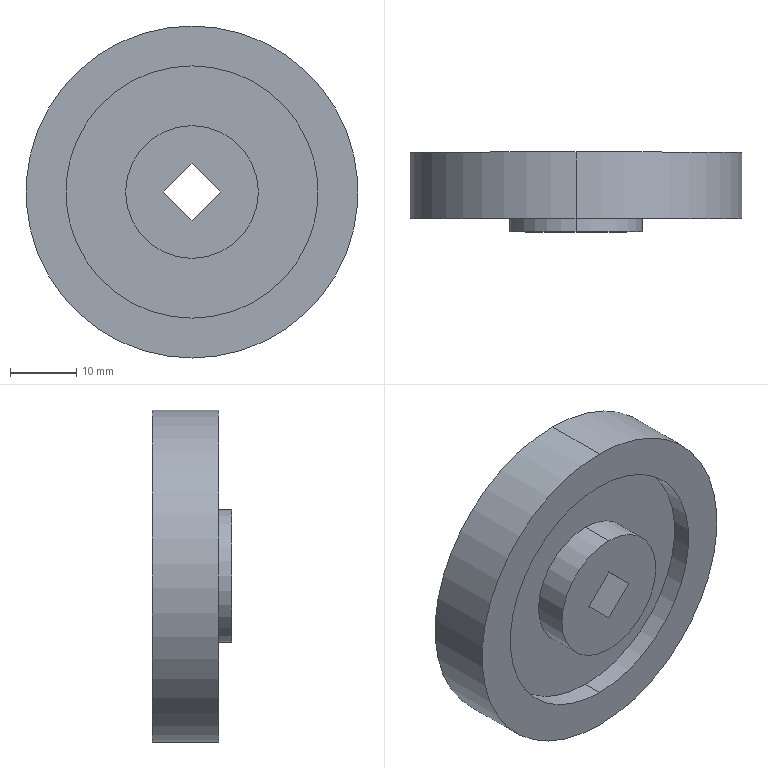Part | SolidWorks | features ICE 3, Extrusion 1 | 1 solid | 20 faces | box 50 x 12 x 50 mm | volume 14912 mm3 | cylinder 10 | plane 10 | commonest cylinder face diameters 20 x4 38 x4 50 x2
STEP:
#1=CARTESIAN_POINT('',(0.,2.,10.));
#2=VERTEX_POINT('',#1);
#3=CARTESIAN_POINT('',(0.,2.,-10.));
#4=VERTEX_POINT('',#3);
#5=CARTESIAN_POINT('',(0.,2.,0.));
#6=DIRECTION('',(0.,1.,0.));
#7=DIRECTION('',(0.,0.,1.));
#8=AXIS2_PLACEMENT_3D('',#5,#6,#7);
#9=CIRCLE('',#8,10.);
#10=EDGE_CURVE('',#2,#4,#9,.T.);
#11=ORIENTED_EDGE('',*,*,#10,.T.);
#12=CARTESIAN_POINT('',(0.,5.,-10.));
#13=VERTEX_POINT('',#12);
#14=CARTESIAN_POINT('',(0.,-7.,-10.));
#15=DIRECTION('',(0.,1.,0.));
#16=VECTOR('',#15,1000.);
#17=LINE('',#14,#16);
#18=EDGE_CURVE('',#4,#13,#17,.T.);
#19=ORIENTED_EDGE('',*,*,#18,.T.);
#20=CARTESIAN_POINT('',(0.,5.,10.));
#21=VERTEX_POINT('',#20);
#22=CARTESIAN_POINT('',(0.,5.,0.));
#23=DIRECTION('',(0.,1.,0.));
#24=DIRECTION('',(0.,0.,1.));
#25=AXIS2_PLACEMENT_3D('',#22,#23,#24);
#26=CIRCLE('',#25,10.);
#27=EDGE_CURVE('',#21,#13,#26,.T.);
#28=ORIENTED_EDGE('',*,*,#27,.F.);
#29=CARTESIAN_POINT('',(0.,-7.,10.));
#30=DIRECTION('',(0.,1.,0.));
#31=VECTOR('',#30,1000.);
#32=LINE('',#29,#31);
#33=EDGE_CURVE('',#2,#21,#32,.T.);
#34=ORIENTED_EDGE('',*,*,#33,.F.);
#35=EDGE_LOOP('',(#11,#19,#28,#34));
#36=FACE_OUTER_BOUND('',#35,.T.);
#37=CARTESIAN_POINT('',(0.,-7.,0.));
#38=DIRECTION('',(0.,1.,0.));
#39=DIRECTION('',(0.,0.,1.));
#40=AXIS2_PLACEMENT_3D('',#37,#38,#39);
#41=CYLINDRICAL_SURFACE('',#40,10.);
#42=ADVANCED_FACE('',(#36),#41,.T.);
#43=CARTESIAN_POINT('',(0.,-7.,10.));
#44=VERTEX_POINT('',#43);
#45=CARTESIAN_POINT('',(0.,-7.,-10.));
#46=VERTEX_POINT('',#45);
#47=CARTESIAN_POINT('',(0.,-7.,0.));
#48=DIRECTION('',(0.,1.,0.));
#49=DIRECTION('',(0.,0.,1.));
#50=AXIS2_PLACEMENT_3D('',#47,#48,#49);
#51=CIRCLE('',#50,10.);
#52=EDGE_CURVE('',#44,#46,#51,.T.);
#53=ORIENTED_EDGE('',*,*,#52,.T.);
#54=CARTESIAN_POINT('',(0.,-2.,-10.));
#55=VERTEX_POINT('',#54);
#56=CARTESIAN_POINT('',(0.,-7.,-10.));
#57=DIRECTION('',(0.,1.,0.));
#58=VECTOR('',#57,1000.);
#59=LINE('',#56,#58);
#60=EDGE_CURVE('',#46,#55,#59,.T.);
#61=ORIENTED_EDGE('',*,*,#60,.T.);
#62=CARTESIAN_POINT('',(0.,-2.,10.));
#63=VERTEX_POINT('',#62);
#64=CARTESIAN_POINT('',(0.,-2.,0.));
#65=DIRECTION('',(0.,1.,0.));
#66=DIRECTION('',(0.,0.,1.));
#67=AXIS2_PLACEMENT_3D('',#64,#65,#66);
#68=CIRCLE('',#67,10.);
#69=EDGE_CURVE('',#63,#55,#68,.T.);
#70=ORIENTED_EDGE('',*,*,#69,.F.);
#71=CARTESIAN_POINT('',(0.,-7.,10.));
#72=DIRECTION('',(0.,1.,0.));
#73=VECTOR('',#72,1000.);
#74=LINE('',#71,#73);
#75=EDGE_CURVE('',#44,#63,#74,.T.);
#76=ORIENTED_EDGE('',*,*,#75,.F.);
#77=EDGE_LOOP('',(#53,#61,#70,#76));
#78=FACE_OUTER_BOUND('',#77,.T.);
#79=CARTESIAN_POINT('',(0.,-7.,0.));
#80=DIRECTION('',(0.,1.,0.));
#81=DIRECTION('',(0.,0.,1.));
#82=AXIS2_PLACEMENT_3D('',#79,#80,#81);
#83=CYLINDRICAL_SURFACE('',#82,10.);
#84=ADVANCED_FACE('',(#78),#83,.T.);
#85=CARTESIAN_POINT('',(0.,5.,-19.));
#86=VERTEX_POINT('',#85);
#87=CARTESIAN_POINT('',(0.,5.,19.));
#88=VERTEX_POINT('',#87);
#89=CARTESIAN_POINT('',(0.,5.,0.));
#90=DIRECTION('',(0.,1.,0.));
#91=DIRECTION('',(0.,0.,1.));
#92=AXIS2_PLACEMENT_3D('',#89,#90,#91);
#93=CIRCLE('',#92,19.);
#94=EDGE_CURVE('',#86,#88,#93,.T.);
#95=ORIENTED_EDGE('',*,*,#94,.T.);
#96=CARTESIAN_POINT('',(0.,2.,19.));
#97=VERTEX_POINT('',#96);
#98=CARTESIAN_POINT('',(0.,5.,19.));
#99=DIRECTION('',(0.,-1.,0.));
#100=VECTOR('',#99,1000.);
#101=LINE('',#98,#100);
#102=EDGE_CURVE('',#88,#97,#101,.T.);
#103=ORIENTED_EDGE('',*,*,#102,.T.);
#104=CARTESIAN_POINT('',(0.,2.,-19.));
#105=VERTEX_POINT('',#104);
#106=CARTESIAN_POINT('',(0.,2.,0.));
#107=DIRECTION('',(0.,1.,0.));
#108=DIRECTION('',(0.,0.,1.));
#109=AXIS2_PLACEMENT_3D('',#106,#107,#108);
#110=CIRCLE('',#109,19.);
#111=EDGE_CURVE('',#105,#97,#110,.T.);
#112=ORIENTED_EDGE('',*,*,#111,.F.);
#113=CARTESIAN_POINT('',(0.,5.,-19.));
#114=DIRECTION('',(0.,-1.,0.));
#115=VECTOR('',#114,1000.);
#116=LINE('',#113,#115);
#117=EDGE_CURVE('',#86,#105,#116,.T.);
#118=ORIENTED_EDGE('',*,*,#117,.F.);
#119=EDGE_LOOP('',(#95,#103,#112,#118));
#120=FACE_OUTER_BOUND('',#119,.T.);
#121=CARTESIAN_POINT('',(0.,5.,0.));
#122=DIRECTION('',(0.,-1.,0.));
#123=DIRECTION('',(0.,0.,-1.));
#124=AXIS2_PLACEMENT_3D('',#121,#122,#123);
#125=CYLINDRICAL_SURFACE('',#124,19.);
#126=ADVANCED_FACE('',(#120),#125,.F.);
#127=CARTESIAN_POINT('',(0.,5.,25.));
#128=VERTEX_POINT('',#127);
#129=CARTESIAN_POINT('',(0.,5.,-25.));
#130=VERTEX_POINT('',#129);
#131=CARTESIAN_POINT('',(0.,5.,0.));
#132=DIRECTION('',(0.,1.,0.));
#133=DIRECTION('',(0.,0.,1.));
#134=AXIS2_PLACEMENT_3D('',#131,#132,#133);
#135=CIRCLE('',#134,25.);
#136=EDGE_CURVE('',#128,#130,#135,.T.);
#137=ORIENTED_EDGE('',*,*,#136,.F.);
#138=CARTESIAN_POINT('',(0.,-5.,25.));
#139=VERTEX_POINT('',#138);
#140=CARTESIAN_POINT('',(0.,5.,25.));
#141=DIRECTION('',(0.,-1.,0.));
#142=VECTOR('',#141,1000.);
#143=LINE('',#140,#142);
#144=EDGE_CURVE('',#128,#139,#143,.T.);
#145=ORIENTED_EDGE('',*,*,#144,.T.);
#146=CARTESIAN_POINT('',(0.,-5.,-25.));
#147=VERTEX_POINT('',#146);
#148=CARTESIAN_POINT('',(0.,-5.,0.));
#149=DIRECTION('',(0.,1.,0.));
#150=DIRECTION('',(0.,0.,1.));
#151=AXIS2_PLACEMENT_3D('',#148,#149,#150);
#152=CIRCLE('',#151,25.);
#153=EDGE_CURVE('',#139,#147,#152,.T.);
#154=ORIENTED_EDGE('',*,*,#153,.T.);
#155=CARTESIAN_POINT('',(0.,5.,-25.));
#156=DIRECTION('',(0.,-1.,0.));
#157=VECTOR('',#156,1000.);
#158=LINE('',#155,#157);
#159=EDGE_CURVE('',#130,#147,#158,.T.);
#160=ORIENTED_EDGE('',*,*,#159,.F.);
#161=EDGE_LOOP('',(#137,#145,#154,#160));
#162=FACE_OUTER_BOUND('',#161,.T.);
#163=CARTESIAN_POINT('',(0.,5.,0.));
#164=DIRECTION('',(0.,-1.,0.));
#165=DIRECTION('',(0.,0.,-1.));
#166=AXIS2_PLACEMENT_3D('',#163,#164,#165);
#167=CYLINDRICAL_SURFACE('',#166,25.);
#168=ADVANCED_FACE('',(#162),#167,.T.);
#169=CARTESIAN_POINT('',(0.,-2.,-19.));
#170=VERTEX_POINT('',#169);
#171=CARTESIAN_POINT('',(0.,-2.,19.));
#172=VERTEX_POINT('',#171);
#173=CARTESIAN_POINT('',(0.,-2.,0.));
#174=DIRECTION('',(0.,1.,0.));
#175=DIRECTION('',(0.,0.,1.));
#176=AXIS2_PLACEMENT_3D('',#173,#174,#175);
#177=CIRCLE('',#176,19.);
#178=EDGE_CURVE('',#170,#172,#177,.T.);
#179=ORIENTED_EDGE('',*,*,#178,.T.);
#180=CARTESIAN_POINT('',(0.,-5.,19.));
#181=VERTEX_POINT('',#180);
#182=CARTESIAN_POINT('',(0.,5.,19.));
#183=DIRECTION('',(0.,-1.,0.));
#184=VECTOR('',#183,1000.);
#185=LINE('',#182,#184);
#186=EDGE_CURVE('',#172,#181,#185,.T.);
#187=ORIENTED_EDGE('',*,*,#186,.T.);
#188=CARTESIAN_POINT('',(0.,-5.,-19.));
#189=VERTEX_POINT('',#188);
#190=CARTESIAN_POINT('',(0.,-5.,0.));
#191=DIRECTION('',(0.,1.,0.));
#192=DIRECTION('',(0.,0.,1.));
#193=AXIS2_PLACEMENT_3D('',#190,#191,#192);
#194=CIRCLE('',#193,19.);
#195=EDGE_CURVE('',#189,#181,#194,.T.);
#196=ORIENTED_EDGE('',*,*,#195,.F.);
#197=CARTESIAN_POINT('',(0.,5.,-19.));
#198=DIRECTION('',(0.,-1.,0.));
#199=VECTOR('',#198,1000.);
#200=LINE('',#197,#199);
#201=EDGE_CURVE('',#170,#189,#200,.T.);
#202=ORIENTED_EDGE('',*,*,#201,.F.);
#203=EDGE_LOOP('',(#179,#187,#196,#202));
#204=FACE_OUTER_BOUND('',#203,.T.);
#205=CARTESIAN_POINT('',(0.,5.,0.));
#206=DIRECTION('',(0.,-1.,0.));
#207=DIRECTION('',(0.,0.,-1.));
#208=AXIS2_PLACEMENT_3D('',#205,#206,#207);
#209=CYLINDRICAL_SURFACE('',#208,19.);
#210=ADVANCED_FACE('',(#204),#209,.F.);
#211=ORIENTED_EDGE('',*,*,#186,.F.);
#212=CARTESIAN_POINT('',(0.,-2.,0.));
#213=DIRECTION('',(0.,1.,0.));
#214=DIRECTION('',(0.,0.,1.));
#215=AXIS2_PLACEMENT_3D('',#212,#213,#214);
#216=CIRCLE('',#215,19.);
#217=EDGE_CURVE('',#172,#170,#216,.T.);
#218=ORIENTED_EDGE('',*,*,#217,.T.);
#219=ORIENTED_EDGE('',*,*,#201,.T.);
#220=CARTESIAN_POINT('',(0.,-5.,0.));
#221=DIRECTION('',(0.,1.,0.));
#222=DIRECTION('',(0.,0.,1.));
#223=AXIS2_PLACEMENT_3D('',#220,#221,#222);
#224=CIRCLE('',#223,19.);
#225=EDGE_CURVE('',#181,#189,#224,.T.);
#226=ORIENTED_EDGE('',*,*,#225,.F.);
#227=EDGE_LOOP('',(#211,#218,#219,#226));
#228=FACE_OUTER_BOUND('',#227,.T.);
#229=CARTESIAN_POINT('',(0.,5.,0.));
#230=DIRECTION('',(0.,-1.,0.));
#231=DIRECTION('',(0.,0.,-1.));
#232=AXIS2_PLACEMENT_3D('',#229,#230,#231);
#233=CYLINDRICAL_SURFACE('',#232,19.);
#234=ADVANCED_FACE('',(#228),#233,.F.);
#235=CARTESIAN_POINT('',(0.,5.,0.));
#236=DIRECTION('',(0.,1.,0.));
#237=DIRECTION('',(0.,0.,1.));
#238=AXIS2_PLACEMENT_3D('',#235,#236,#237);
#239=CIRCLE('',#238,25.);
#240=EDGE_CURVE('',#130,#128,#239,.T.);
#241=ORIENTED_EDGE('',*,*,#240,.T.);
#242=ORIENTED_EDGE('',*,*,#136,.T.);
#243=EDGE_LOOP('',(#241,#242));
#244=FACE_OUTER_BOUND('',#243,.T.);
#245=ORIENTED_EDGE('',*,*,#94,.F.);
#246=CARTESIAN_POINT('',(0.,5.,0.));
#247=DIRECTION('',(0.,1.,0.));
#248=DIRECTION('',(0.,0.,1.));
#249=AXIS2_PLACEMENT_3D('',#246,#247,#248);
#250=CIRCLE('',#249,19.);
#251=EDGE_CURVE('',#88,#86,#250,.T.);
#252=ORIENTED_EDGE('',*,*,#251,.F.);
#253=EDGE_LOOP('',(#245,#252));
#254=FACE_BOUND('',#253,.T.);
#255=CARTESIAN_POINT('',(0.,5.,0.));
#256=DIRECTION('',(0.,1.,0.));
#257=DIRECTION('',(0.,0.,1.));
#258=AXIS2_PLACEMENT_3D('',#255,#256,#257);
#259=PLANE('',#258);
#260=ADVANCED_FACE('',(#244,#254),#259,.T.);
#261=CARTESIAN_POINT('',(0.,-5.,0.));
#262=DIRECTION('',(0.,1.,0.));
#263=DIRECTION('',(0.,0.,1.));
#264=AXIS2_PLACEMENT_3D('',#261,#262,#263);
#265=CIRCLE('',#264,25.);
#266=EDGE_CURVE('',#147,#139,#265,.T.);
#267=ORIENTED_EDGE('',*,*,#266,.F.);
#268=ORIENTED_EDGE('',*,*,#153,.F.);
#269=EDGE_LOOP('',(#267,#268));
#270=FACE_OUTER_BOUND('',#269,.T.);
#271=ORIENTED_EDGE('',*,*,#195,.T.);
#272=ORIENTED_EDGE('',*,*,#225,.T.);
#273=EDGE_LOOP('',(#271,#272));
#274=FACE_BOUND('',#273,.T.);
#275=CARTESIAN_POINT('',(0.,-5.,0.));
#276=DIRECTION('',(0.,1.,0.));
#277=DIRECTION('',(0.,0.,1.));
#278=AXIS2_PLACEMENT_3D('',#275,#276,#277);
#279=PLANE('',#278);
#280=ADVANCED_FACE('',(#270,#274),#279,.F.);
#281=ORIENTED_EDGE('',*,*,#144,.F.);
#282=ORIENTED_EDGE('',*,*,#240,.F.);
#283=ORIENTED_EDGE('',*,*,#159,.T.);
#284=ORIENTED_EDGE('',*,*,#266,.T.);
#285=EDGE_LOOP('',(#281,#282,#283,#284));
#286=FACE_OUTER_BOUND('',#285,.T.);
#287=CARTESIAN_POINT('',(0.,5.,0.));
#288=DIRECTION('',(0.,-1.,0.));
#289=DIRECTION('',(0.,0.,-1.));
#290=AXIS2_PLACEMENT_3D('',#287,#288,#289);
#291=CYLINDRICAL_SURFACE('',#290,25.);
#292=ADVANCED_FACE('',(#286),#291,.T.);
#293=ORIENTED_EDGE('',*,*,#102,.F.);
#294=ORIENTED_EDGE('',*,*,#251,.T.);
#295=ORIENTED_EDGE('',*,*,#117,.T.);
#296=CARTESIAN_POINT('',(0.,2.,0.));
#297=DIRECTION('',(0.,1.,0.));
#298=DIRECTION('',(0.,0.,1.));
#299=AXIS2_PLACEMENT_3D('',#296,#297,#298);
#300=CIRCLE('',#299,19.);
#301=EDGE_CURVE('',#97,#105,#300,.T.);
#302=ORIENTED_EDGE('',*,*,#301,.F.);
#303=EDGE_LOOP('',(#293,#294,#295,#302));
#304=FACE_OUTER_BOUND('',#303,.T.);
#305=CARTESIAN_POINT('',(0.,5.,0.));
#306=DIRECTION('',(0.,-1.,0.));
#307=DIRECTION('',(0.,0.,-1.));
#308=AXIS2_PLACEMENT_3D('',#305,#306,#307);
#309=CYLINDRICAL_SURFACE('',#308,19.);
#310=ADVANCED_FACE('',(#304),#309,.F.);
#311=ORIENTED_EDGE('',*,*,#111,.T.);
#312=ORIENTED_EDGE('',*,*,#301,.T.);
#313=EDGE_LOOP('',(#311,#312));
#314=FACE_OUTER_BOUND('',#313,.T.);
#315=ORIENTED_EDGE('',*,*,#10,.F.);
#316=CARTESIAN_POINT('',(0.,2.,0.));
#317=DIRECTION('',(0.,1.,0.));
#318=DIRECTION('',(0.,0.,1.));
#319=AXIS2_PLACEMENT_3D('',#316,#317,#318);
#320=CIRCLE('',#319,10.);
#321=EDGE_CURVE('',#4,#2,#320,.T.);
#322=ORIENTED_EDGE('',*,*,#321,.F.);
#323=EDGE_LOOP('',(#315,#322));
#324=FACE_BOUND('',#323,.T.);
#325=CARTESIAN_POINT('',(0.,2.,0.));
#326=DIRECTION('',(0.,1.,0.));
#327=DIRECTION('',(0.,0.,1.));
#328=AXIS2_PLACEMENT_3D('',#325,#326,#327);
#329=PLANE('',#328);
#330=ADVANCED_FACE('',(#314,#324),#329,.T.);
#331=ORIENTED_EDGE('',*,*,#178,.F.);
#332=ORIENTED_EDGE('',*,*,#217,.F.);
#333=EDGE_LOOP('',(#331,#332));
#334=FACE_OUTER_BOUND('',#333,.T.);
#335=ORIENTED_EDGE('',*,*,#69,.T.);
#336=CARTESIAN_POINT('',(0.,-2.,0.));
#337=DIRECTION('',(0.,1.,0.));
#338=DIRECTION('',(0.,0.,1.));
#339=AXIS2_PLACEMENT_3D('',#336,#337,#338);
#340=CIRCLE('',#339,10.);
#341=EDGE_CURVE('',#55,#63,#340,.T.);
#342=ORIENTED_EDGE('',*,*,#341,.T.);
#343=EDGE_LOOP('',(#335,#342));
#344=FACE_BOUND('',#343,.T.);
#345=CARTESIAN_POINT('',(0.,-2.,0.));
#346=DIRECTION('',(0.,1.,0.));
#347=DIRECTION('',(0.,0.,1.));
#348=AXIS2_PLACEMENT_3D('',#345,#346,#347);
#349=PLANE('',#348);
#350=ADVANCED_FACE('',(#334,#344),#349,.F.);
#351=CARTESIAN_POINT('',(0.,-7.,-4.243));
#352=VERTEX_POINT('',#351);
#353=CARTESIAN_POINT('',(4.243,-7.,0.));
#354=VERTEX_POINT('',#353);
#355=CARTESIAN_POINT('',(0.,-7.,-4.243));
#356=DIRECTION('',(0.7071,0.,0.7071));
#357=VECTOR('',#356,1000.);
#358=LINE('',#355,#357);
#359=EDGE_CURVE('',#352,#354,#358,.T.);
#360=ORIENTED_EDGE('',*,*,#359,.F.);
#361=CARTESIAN_POINT('',(-4.243,-7.,0.));
#362=VERTEX_POINT('',#361);
#363=CARTESIAN_POINT('',(-4.243,-7.,0.));
#364=DIRECTION('',(0.7071,0.,-0.7071));
#365=VECTOR('',#364,1000.);
#366=LINE('',#363,#365);
#367=EDGE_CURVE('',#362,#352,#366,.T.);
#368=ORIENTED_EDGE('',*,*,#367,.F.);
#369=CARTESIAN_POINT('',(0.,-7.,4.243));
#370=VERTEX_POINT('',#369);
#371=CARTESIAN_POINT('',(-4.243,-7.,0.));
#372=DIRECTION('',(-0.7071,0.,-0.7071));
#373=VECTOR('',#372,1000.);
#374=LINE('',#371,#373);
#375=EDGE_CURVE('',#370,#362,#374,.T.);
#376=ORIENTED_EDGE('',*,*,#375,.F.);
#377=CARTESIAN_POINT('',(0.,-7.,4.243));
#378=DIRECTION('',(-0.7071,0.,0.7071));
#379=VECTOR('',#378,1000.);
#380=LINE('',#377,#379);
#381=EDGE_CURVE('',#354,#370,#380,.T.);
#382=ORIENTED_EDGE('',*,*,#381,.F.);
#383=EDGE_LOOP('',(#360,#368,#376,#382));
#384=FACE_BOUND('',#383,.T.);
#385=ORIENTED_EDGE('',*,*,#52,.F.);
#386=CARTESIAN_POINT('',(0.,-7.,0.));
#387=DIRECTION('',(0.,1.,0.));
#388=DIRECTION('',(0.,0.,1.));
#389=AXIS2_PLACEMENT_3D('',#386,#387,#388);
#390=CIRCLE('',#389,10.);
#391=EDGE_CURVE('',#46,#44,#390,.T.);
#392=ORIENTED_EDGE('',*,*,#391,.F.);
#393=EDGE_LOOP('',(#385,#392));
#394=FACE_OUTER_BOUND('',#393,.T.);
#395=CARTESIAN_POINT('',(0.,-7.,0.));
#396=DIRECTION('',(0.,1.,0.));
#397=DIRECTION('',(0.,0.,1.));
#398=AXIS2_PLACEMENT_3D('',#395,#396,#397);
#399=PLANE('',#398);
#400=ADVANCED_FACE('',(#384,#394),#399,.F.);
#401=ORIENTED_EDGE('',*,*,#60,.F.);
#402=ORIENTED_EDGE('',*,*,#391,.T.);
#403=ORIENTED_EDGE('',*,*,#75,.T.);
#404=ORIENTED_EDGE('',*,*,#341,.F.);
#405=EDGE_LOOP('',(#401,#402,#403,#404));
#406=FACE_OUTER_BOUND('',#405,.T.);
#407=CARTESIAN_POINT('',(0.,-7.,0.));
#408=DIRECTION('',(0.,1.,0.));
#409=DIRECTION('',(0.,0.,1.));
#410=AXIS2_PLACEMENT_3D('',#407,#408,#409);
#411=CYLINDRICAL_SURFACE('',#410,10.);
#412=ADVANCED_FACE('',(#406),#411,.T.);
#413=ORIENTED_EDGE('',*,*,#18,.F.);
#414=ORIENTED_EDGE('',*,*,#321,.T.);
#415=ORIENTED_EDGE('',*,*,#33,.T.);
#416=CARTESIAN_POINT('',(0.,5.,0.));
#417=DIRECTION('',(0.,1.,0.));
#418=DIRECTION('',(0.,0.,1.));
#419=AXIS2_PLACEMENT_3D('',#416,#417,#418);
#420=CIRCLE('',#419,10.);
#421=EDGE_CURVE('',#13,#21,#420,.T.);
#422=ORIENTED_EDGE('',*,*,#421,.F.);
#423=EDGE_LOOP('',(#413,#414,#415,#422));
#424=FACE_OUTER_BOUND('',#423,.T.);
#425=CARTESIAN_POINT('',(0.,-7.,0.));
#426=DIRECTION('',(0.,1.,0.));
#427=DIRECTION('',(0.,0.,1.));
#428=AXIS2_PLACEMENT_3D('',#425,#426,#427);
#429=CYLINDRICAL_SURFACE('',#428,10.);
#430=ADVANCED_FACE('',(#424),#429,.T.);
#431=CARTESIAN_POINT('',(0.,5.,-4.243));
#432=VERTEX_POINT('',#431);
#433=CARTESIAN_POINT('',(-4.243,5.,0.));
#434=VERTEX_POINT('',#433);
#435=CARTESIAN_POINT('',(-2.121,5.,-2.121));
#436=DIRECTION('',(-0.7071,0.,0.7071));
#437=VECTOR('',#436,1000.);
#438=LINE('',#435,#437);
#439=EDGE_CURVE('',#432,#434,#438,.T.);
#440=ORIENTED_EDGE('',*,*,#439,.F.);
#441=CARTESIAN_POINT('',(4.243,5.,0.));
#442=VERTEX_POINT('',#441);
#443=CARTESIAN_POINT('',(2.121,5.,-2.121));
#444=DIRECTION('',(-0.7071,0.,-0.7071));
#445=VECTOR('',#444,1000.);
#446=LINE('',#443,#445);
#447=EDGE_CURVE('',#442,#432,#446,.T.);
#448=ORIENTED_EDGE('',*,*,#447,.F.);
#449=CARTESIAN_POINT('',(0.,5.,4.243));
#450=VERTEX_POINT('',#449);
#451=CARTESIAN_POINT('',(2.121,5.,2.121));
#452=DIRECTION('',(0.7071,0.,-0.7071));
#453=VECTOR('',#452,1000.);
#454=LINE('',#451,#453);
#455=EDGE_CURVE('',#450,#442,#454,.T.);
#456=ORIENTED_EDGE('',*,*,#455,.F.);
#457=CARTESIAN_POINT('',(-2.121,5.,2.121));
#458=DIRECTION('',(0.7071,0.,0.7071));
#459=VECTOR('',#458,1000.);
#460=LINE('',#457,#459);
#461=EDGE_CURVE('',#434,#450,#460,.T.);
#462=ORIENTED_EDGE('',*,*,#461,.F.);
#463=EDGE_LOOP('',(#440,#448,#456,#462));
#464=FACE_BOUND('',#463,.T.);
#465=ORIENTED_EDGE('',*,*,#27,.T.);
#466=ORIENTED_EDGE('',*,*,#421,.T.);
#467=EDGE_LOOP('',(#465,#466));
#468=FACE_OUTER_BOUND('',#467,.T.);
#469=CARTESIAN_POINT('',(0.,5.,0.));
#470=DIRECTION('',(0.,1.,0.));
#471=DIRECTION('',(0.,0.,1.));
#472=AXIS2_PLACEMENT_3D('',#469,#470,#471);
#473=PLANE('',#472);
#474=ADVANCED_FACE('',(#464,#468),#473,.T.);
#475=ORIENTED_EDGE('',*,*,#439,.T.);
#476=CARTESIAN_POINT('',(-4.243,43.,0.));
#477=DIRECTION('',(0.,-1.,0.));
#478=VECTOR('',#477,1000.);
#479=LINE('',#476,#478);
#480=EDGE_CURVE('',#434,#362,#479,.T.);
#481=ORIENTED_EDGE('',*,*,#480,.T.);
#482=ORIENTED_EDGE('',*,*,#367,.T.);
#483=CARTESIAN_POINT('',(0.,43.,-4.243));
#484=DIRECTION('',(0.,-1.,0.));
#485=VECTOR('',#484,1000.);
#486=LINE('',#483,#485);
#487=EDGE_CURVE('',#432,#352,#486,.T.);
#488=ORIENTED_EDGE('',*,*,#487,.F.);
#489=EDGE_LOOP('',(#475,#481,#482,#488));
#490=FACE_OUTER_BOUND('',#489,.T.);
#491=CARTESIAN_POINT('',(-4.243,43.,0.));
#492=DIRECTION('',(-0.7071,0.,-0.7071));
#493=DIRECTION('',(-0.7071,0.,0.7071));
#494=AXIS2_PLACEMENT_3D('',#491,#492,#493);
#495=PLANE('',#494);
#496=ADVANCED_FACE('',(#490),#495,.F.);
#497=ORIENTED_EDGE('',*,*,#461,.T.);
#498=CARTESIAN_POINT('',(0.,43.,4.243));
#499=DIRECTION('',(0.,-1.,0.));
#500=VECTOR('',#499,1000.);
#501=LINE('',#498,#500);
#502=EDGE_CURVE('',#450,#370,#501,.T.);
#503=ORIENTED_EDGE('',*,*,#502,.T.);
#504=ORIENTED_EDGE('',*,*,#375,.T.);
#505=ORIENTED_EDGE('',*,*,#480,.F.);
#506=EDGE_LOOP('',(#497,#503,#504,#505));
#507=FACE_OUTER_BOUND('',#506,.T.);
#508=CARTESIAN_POINT('',(-4.243,43.,0.));
#509=DIRECTION('',(-0.7071,0.,0.7071));
#510=DIRECTION('',(0.7071,0.,0.7071));
#511=AXIS2_PLACEMENT_3D('',#508,#509,#510);
#512=PLANE('',#511);
#513=ADVANCED_FACE('',(#507),#512,.F.);
#514=ORIENTED_EDGE('',*,*,#455,.T.);
#515=CARTESIAN_POINT('',(4.243,43.,0.));
#516=DIRECTION('',(0.,-1.,0.));
#517=VECTOR('',#516,1000.);
#518=LINE('',#515,#517);
#519=EDGE_CURVE('',#442,#354,#518,.T.);
#520=ORIENTED_EDGE('',*,*,#519,.T.);
#521=ORIENTED_EDGE('',*,*,#381,.T.);
#522=ORIENTED_EDGE('',*,*,#502,.F.);
#523=EDGE_LOOP('',(#514,#520,#521,#522));
#524=FACE_OUTER_BOUND('',#523,.T.);
#525=CARTESIAN_POINT('',(0.,43.,4.243));
#526=DIRECTION('',(0.7071,0.,0.7071));
#527=DIRECTION('',(0.7071,0.,-0.7071));
#528=AXIS2_PLACEMENT_3D('',#525,#526,#527);
#529=PLANE('',#528);
#530=ADVANCED_FACE('',(#524),#529,.F.);
#531=ORIENTED_EDGE('',*,*,#447,.T.);
#532=ORIENTED_EDGE('',*,*,#487,.T.);
#533=ORIENTED_EDGE('',*,*,#359,.T.);
#534=ORIENTED_EDGE('',*,*,#519,.F.);
#535=EDGE_LOOP('',(#531,#532,#533,#534));
#536=FACE_OUTER_BOUND('',#535,.T.);
#537=CARTESIAN_POINT('',(0.,43.,-4.243));
#538=DIRECTION('',(0.7071,0.,-0.7071));
#539=DIRECTION('',(-0.7071,0.,-0.7071));
#540=AXIS2_PLACEMENT_3D('',#537,#538,#539);
#541=PLANE('',#540);
#542=ADVANCED_FACE('',(#536),#541,.F.);
#543=CLOSED_SHELL('',(#42,#84,#126,#168,#210,#234,#260,#280,#292,#310,#330,#350,#400,#412,#430,#474,#496,#513,#530,#542));
#544=MANIFOLD_SOLID_BREP('',#543);
#545=CARTESIAN_POINT('',(0.,0.,0.));
#546=DIRECTION('',(0.,0.,1.));
#547=DIRECTION('',(1.,0.,0.));
#548=AXIS2_PLACEMENT_3D('',#545,#546,#547);
#549=(LENGTH_UNIT()NAMED_UNIT(*)SI_UNIT(.MILLI.,.METRE.));
#550=UNCERTAINTY_MEASURE_WITH_UNIT(LENGTH_MEASURE(0.00001),#549,'','');
#551=(NAMED_UNIT(*)PLANE_ANGLE_UNIT()SI_UNIT($,.RADIAN.));
#552=(NAMED_UNIT(*)SI_UNIT($,.STERADIAN.)SOLID_ANGLE_UNIT());
#553=(GEOMETRIC_REPRESENTATION_CONTEXT(3)GLOBAL_UNCERTAINTY_ASSIGNED_CONTEXT((#550))GLOBAL_UNIT_ASSIGNED_CONTEXT((#549,#551,#552))REPRESENTATION_CONTEXT('',''));
#554=ADVANCED_BREP_SHAPE_REPRESENTATION('',(#544,#548),#553);